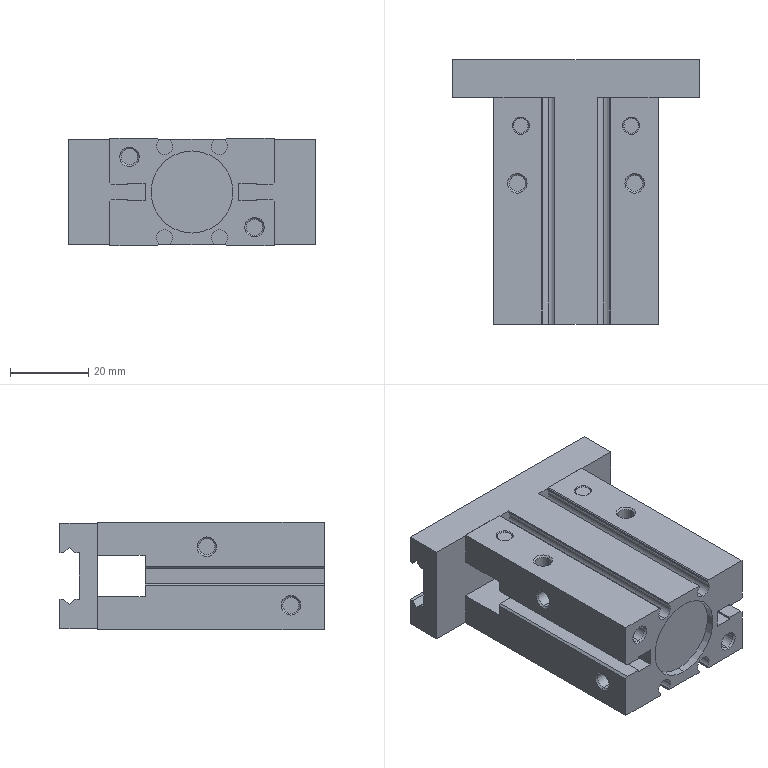Part | SolidWorks | features BaseBody 1 | 1 solid | 157 faces | box 63 x 67.6 x 27.5 mm | volume 65251 mm3 | plane 85 | cylinder 44 | cone 28 | commonest cylinder face diameters 4.134 x20 3.8 x8 4 x8 4.2 x6 21 x2